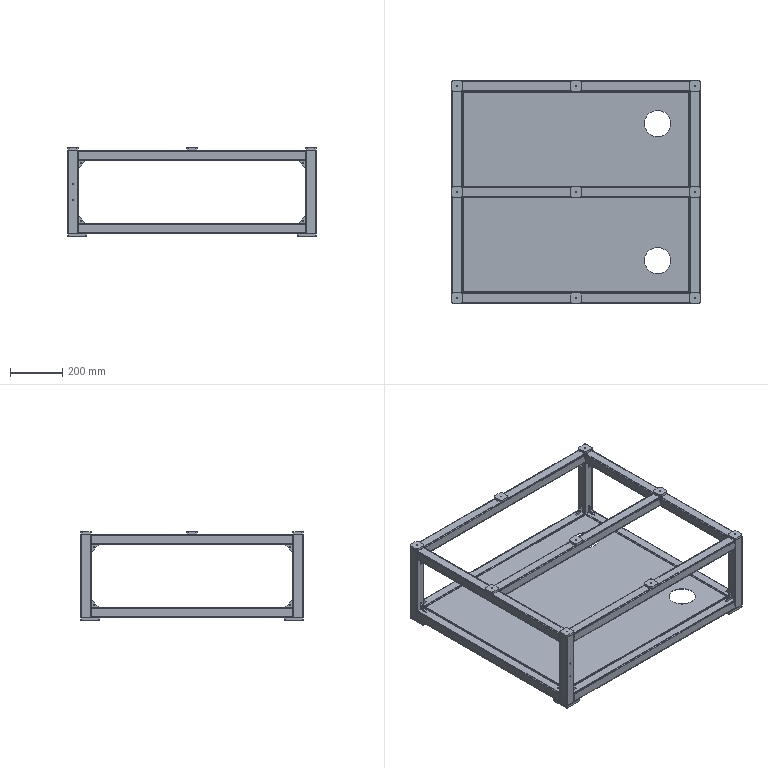Part | SolidWorks | features Fillet 10, Gusset 8, HoleWzd 8, WeldCornerFeat 8, MirrorSolid 4, ICE 3, 3DProfileFeature 1, EdgeFlange 1, FlatPattern 1, MirrorPattern 1, SMBaseFlange 1, SheetMetal 1, WeldMemberFeat 1, WeldmentFeature 1 | 43 solids | 605 faces | box 950 x 850 x 340 mm | volume 4003537 mm3 | plane 317 | cylinder 280 | spline 8 | commonest cylinder face diameters 5 x72 8 x68 4 x56 10 x36 4.2 x32 10.2 x8